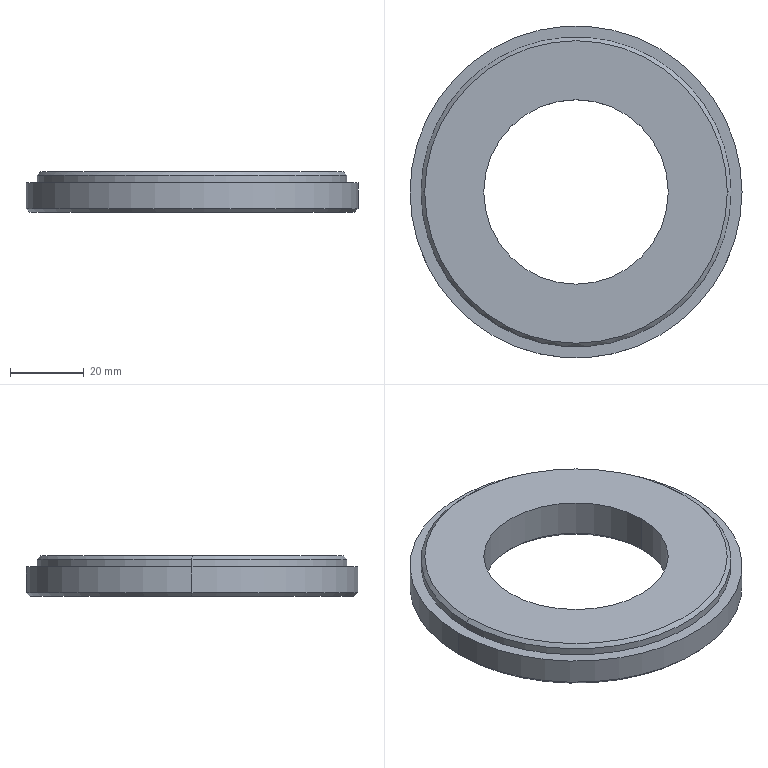Part | SolidWorks | features Chamfer 2, HoleWzd 1, ICE 1, Revolution 1 | 1 solid | 51 faces | box 90 x 90 x 11 mm | volume 45138 mm3 | cone 30 | cylinder 18 | plane 3 | commonest cylinder face diameters 3.3 x12 50 x2 84 x2 90 x2
STEP:
#1=CARTESIAN_POINT('',(-44.,0.,-11.));
#2=VERTEX_POINT('',#1);
#3=CARTESIAN_POINT('',(44.,0.,-11.));
#4=VERTEX_POINT('',#3);
#5=CARTESIAN_POINT('',(0.,0.,-11.));
#6=DIRECTION('',(0.,0.,-1.));
#7=DIRECTION('',(-1.,0.,0.));
#8=AXIS2_PLACEMENT_3D('',#5,#6,#7);
#9=CIRCLE('',#8,44.);
#10=EDGE_CURVE('',#2,#4,#9,.T.);
#11=ORIENTED_EDGE('',*,*,#10,.F.);
#12=CARTESIAN_POINT('',(-45.,0.,-10.));
#13=VERTEX_POINT('',#12);
#14=CARTESIAN_POINT('',(-45.,0.,-10.));
#15=DIRECTION('',(-0.7071,0.,0.7071));
#16=VECTOR('',#15,1000.);
#17=LINE('',#14,#16);
#18=EDGE_CURVE('',#2,#13,#17,.T.);
#19=ORIENTED_EDGE('',*,*,#18,.T.);
#20=CARTESIAN_POINT('',(45.,0.,-10.));
#21=VERTEX_POINT('',#20);
#22=CARTESIAN_POINT('',(0.,0.,-10.));
#23=DIRECTION('',(0.,0.,1.));
#24=DIRECTION('',(-1.,0.,0.));
#25=AXIS2_PLACEMENT_3D('',#22,#23,#24);
#26=CIRCLE('',#25,45.);
#27=EDGE_CURVE('',#21,#13,#26,.T.);
#28=ORIENTED_EDGE('',*,*,#27,.F.);
#29=CARTESIAN_POINT('',(45.,0.,-10.));
#30=DIRECTION('',(0.7071,0.,0.7071));
#31=VECTOR('',#30,1000.);
#32=LINE('',#29,#31);
#33=EDGE_CURVE('',#4,#21,#32,.T.);
#34=ORIENTED_EDGE('',*,*,#33,.F.);
#35=EDGE_LOOP('',(#11,#19,#28,#34));
#36=FACE_OUTER_BOUND('',#35,.T.);
#37=CARTESIAN_POINT('',(0.,0.,-10.));
#38=DIRECTION('',(0.,0.,1.));
#39=DIRECTION('',(1.,0.,0.));
#40=AXIS2_PLACEMENT_3D('',#37,#38,#39);
#41=CONICAL_SURFACE('',#40,45.,0.7854);
#42=ADVANCED_FACE('',(#36),#41,.T.);
#43=CARTESIAN_POINT('',(25.,0.,-10.));
#44=VERTEX_POINT('',#43);
#45=CARTESIAN_POINT('',(-25.,0.,-10.));
#46=VERTEX_POINT('',#45);
#47=CARTESIAN_POINT('',(0.,0.,-10.));
#48=DIRECTION('',(0.,0.,-1.));
#49=DIRECTION('',(-1.,0.,0.));
#50=AXIS2_PLACEMENT_3D('',#47,#48,#49);
#51=CIRCLE('',#50,25.);
#52=EDGE_CURVE('',#44,#46,#51,.T.);
#53=ORIENTED_EDGE('',*,*,#52,.F.);
#54=CARTESIAN_POINT('',(26.,0.,-11.));
#55=VERTEX_POINT('',#54);
#56=CARTESIAN_POINT('',(26.,0.,-11.));
#57=DIRECTION('',(0.7071,0.,-0.7071));
#58=VECTOR('',#57,1000.);
#59=LINE('',#56,#58);
#60=EDGE_CURVE('',#44,#55,#59,.T.);
#61=ORIENTED_EDGE('',*,*,#60,.T.);
#62=CARTESIAN_POINT('',(-26.,0.,-11.));
#63=VERTEX_POINT('',#62);
#64=CARTESIAN_POINT('',(0.,0.,-11.));
#65=DIRECTION('',(0.,0.,1.));
#66=DIRECTION('',(-1.,0.,0.));
#67=AXIS2_PLACEMENT_3D('',#64,#65,#66);
#68=CIRCLE('',#67,26.);
#69=EDGE_CURVE('',#63,#55,#68,.T.);
#70=ORIENTED_EDGE('',*,*,#69,.F.);
#71=CARTESIAN_POINT('',(-26.,0.,-11.));
#72=DIRECTION('',(-0.7071,0.,-0.7071));
#73=VECTOR('',#72,1000.);
#74=LINE('',#71,#73);
#75=EDGE_CURVE('',#46,#63,#74,.T.);
#76=ORIENTED_EDGE('',*,*,#75,.F.);
#77=EDGE_LOOP('',(#53,#61,#70,#76));
#78=FACE_OUTER_BOUND('',#77,.T.);
#79=CARTESIAN_POINT('',(0.,0.,-11.));
#80=DIRECTION('',(0.,0.,-1.));
#81=DIRECTION('',(-1.,0.,0.));
#82=AXIS2_PLACEMENT_3D('',#79,#80,#81);
#83=CONICAL_SURFACE('',#82,26.,0.7854);
#84=ADVANCED_FACE('',(#78),#83,.F.);
#85=CARTESIAN_POINT('',(41.,0.,0.));
#86=VERTEX_POINT('',#85);
#87=CARTESIAN_POINT('',(-41.,0.,0.));
#88=VERTEX_POINT('',#87);
#89=CARTESIAN_POINT('',(0.,0.,0.));
#90=DIRECTION('',(0.,0.,1.));
#91=DIRECTION('',(1.,0.,0.));
#92=AXIS2_PLACEMENT_3D('',#89,#90,#91);
#93=CIRCLE('',#92,41.);
#94=EDGE_CURVE('',#86,#88,#93,.T.);
#95=ORIENTED_EDGE('',*,*,#94,.F.);
#96=CARTESIAN_POINT('',(42.,0.,-1.));
#97=VERTEX_POINT('',#96);
#98=CARTESIAN_POINT('',(41.,0.,0.));
#99=DIRECTION('',(0.7071,0.,-0.7071));
#100=VECTOR('',#99,1000.);
#101=LINE('',#98,#100);
#102=EDGE_CURVE('',#86,#97,#101,.T.);
#103=ORIENTED_EDGE('',*,*,#102,.T.);
#104=CARTESIAN_POINT('',(-42.,0.,-1.));
#105=VERTEX_POINT('',#104);
#106=CARTESIAN_POINT('',(0.,0.,-1.));
#107=DIRECTION('',(0.,0.,-1.));
#108=DIRECTION('',(1.,0.,0.));
#109=AXIS2_PLACEMENT_3D('',#106,#107,#108);
#110=CIRCLE('',#109,42.);
#111=EDGE_CURVE('',#105,#97,#110,.T.);
#112=ORIENTED_EDGE('',*,*,#111,.F.);
#113=CARTESIAN_POINT('',(-41.,0.,0.));
#114=DIRECTION('',(-0.7071,0.,-0.7071));
#115=VECTOR('',#114,1000.);
#116=LINE('',#113,#115);
#117=EDGE_CURVE('',#88,#105,#116,.T.);
#118=ORIENTED_EDGE('',*,*,#117,.F.);
#119=EDGE_LOOP('',(#95,#103,#112,#118));
#120=FACE_OUTER_BOUND('',#119,.T.);
#121=CARTESIAN_POINT('',(0.,0.,0.));
#122=DIRECTION('',(0.,0.,-1.));
#123=DIRECTION('',(-1.,0.,0.));
#124=AXIS2_PLACEMENT_3D('',#121,#122,#123);
#125=CONICAL_SURFACE('',#124,41.,0.7854);
#126=ADVANCED_FACE('',(#120),#125,.T.);
#127=CARTESIAN_POINT('',(1.65,37.,-10.625));
#128=VERTEX_POINT('',#127);
#129=CARTESIAN_POINT('',(-1.65,37.,-10.625));
#130=VERTEX_POINT('',#129);
#131=CARTESIAN_POINT('',(0.,37.,-10.625));
#132=DIRECTION('',(0.,0.,-1.));
#133=DIRECTION('',(-1.,0.,0.));
#134=AXIS2_PLACEMENT_3D('',#131,#132,#133);
#135=CIRCLE('',#134,1.65);
#136=EDGE_CURVE('',#128,#130,#135,.T.);
#137=ORIENTED_EDGE('',*,*,#136,.F.);
#138=CARTESIAN_POINT('',(2.025,37.,-11.));
#139=VERTEX_POINT('',#138);
#140=CARTESIAN_POINT('',(1.65,37.,-10.625));
#141=DIRECTION('',(0.7071,0.,-0.7071));
#142=VECTOR('',#141,1000.);
#143=LINE('',#140,#142);
#144=EDGE_CURVE('',#128,#139,#143,.T.);
#145=ORIENTED_EDGE('',*,*,#144,.T.);
#146=CARTESIAN_POINT('',(-2.025,37.,-11.));
#147=VERTEX_POINT('',#146);
#148=CARTESIAN_POINT('',(0.,37.,-11.));
#149=DIRECTION('',(0.,0.,1.));
#150=DIRECTION('',(-1.,0.,0.));
#151=AXIS2_PLACEMENT_3D('',#148,#149,#150);
#152=CIRCLE('',#151,2.025);
#153=EDGE_CURVE('',#147,#139,#152,.T.);
#154=ORIENTED_EDGE('',*,*,#153,.F.);
#155=CARTESIAN_POINT('',(-1.65,37.,-10.625));
#156=DIRECTION('',(-0.7071,0.,-0.7071));
#157=VECTOR('',#156,1000.);
#158=LINE('',#155,#157);
#159=EDGE_CURVE('',#130,#147,#158,.T.);
#160=ORIENTED_EDGE('',*,*,#159,.F.);
#161=EDGE_LOOP('',(#137,#145,#154,#160));
#162=FACE_OUTER_BOUND('',#161,.T.);
#163=CARTESIAN_POINT('',(0.,37.,-10.625));
#164=DIRECTION('',(0.,0.,-1.));
#165=DIRECTION('',(-1.,0.,0.));
#166=AXIS2_PLACEMENT_3D('',#163,#164,#165);
#167=CONICAL_SURFACE('',#166,1.65,0.7854);
#168=ADVANCED_FACE('',(#162),#167,.F.);
#169=CARTESIAN_POINT('',(33.693,18.5,-10.625));
#170=VERTEX_POINT('',#169);
#171=CARTESIAN_POINT('',(30.393,18.5,-10.625));
#172=VERTEX_POINT('',#171);
#173=CARTESIAN_POINT('',(32.043,18.5,-10.625));
#174=DIRECTION('',(0.,0.,-1.));
#175=DIRECTION('',(-1.,0.,0.));
#176=AXIS2_PLACEMENT_3D('',#173,#174,#175);
#177=CIRCLE('',#176,1.65);
#178=EDGE_CURVE('',#170,#172,#177,.T.);
#179=ORIENTED_EDGE('',*,*,#178,.F.);
#180=CARTESIAN_POINT('',(34.068,18.5,-11.));
#181=VERTEX_POINT('',#180);
#182=CARTESIAN_POINT('',(33.693,18.5,-10.625));
#183=DIRECTION('',(0.7071,0.,-0.7071));
#184=VECTOR('',#183,1000.);
#185=LINE('',#182,#184);
#186=EDGE_CURVE('',#170,#181,#185,.T.);
#187=ORIENTED_EDGE('',*,*,#186,.T.);
#188=CARTESIAN_POINT('',(30.018,18.5,-11.));
#189=VERTEX_POINT('',#188);
#190=CARTESIAN_POINT('',(32.043,18.5,-11.));
#191=DIRECTION('',(0.,0.,1.));
#192=DIRECTION('',(-1.,0.,0.));
#193=AXIS2_PLACEMENT_3D('',#190,#191,#192);
#194=CIRCLE('',#193,2.025);
#195=EDGE_CURVE('',#189,#181,#194,.T.);
#196=ORIENTED_EDGE('',*,*,#195,.F.);
#197=CARTESIAN_POINT('',(30.393,18.5,-10.625));
#198=DIRECTION('',(-0.7071,0.,-0.7071));
#199=VECTOR('',#198,1000.);
#200=LINE('',#197,#199);
#201=EDGE_CURVE('',#172,#189,#200,.T.);
#202=ORIENTED_EDGE('',*,*,#201,.F.);
#203=EDGE_LOOP('',(#179,#187,#196,#202));
#204=FACE_OUTER_BOUND('',#203,.T.);
#205=CARTESIAN_POINT('',(32.043,18.5,-10.625));
#206=DIRECTION('',(0.,0.,-1.));
#207=DIRECTION('',(-1.,0.,0.));
#208=AXIS2_PLACEMENT_3D('',#205,#206,#207);
#209=CONICAL_SURFACE('',#208,1.65,0.7854);
#210=ADVANCED_FACE('',(#204),#209,.F.);
#211=CARTESIAN_POINT('',(33.693,-18.5,-10.625));
#212=VERTEX_POINT('',#211);
#213=CARTESIAN_POINT('',(30.393,-18.5,-10.625));
#214=VERTEX_POINT('',#213);
#215=CARTESIAN_POINT('',(32.043,-18.5,-10.625));
#216=DIRECTION('',(0.,0.,-1.));
#217=DIRECTION('',(-1.,0.,0.));
#218=AXIS2_PLACEMENT_3D('',#215,#216,#217);
#219=CIRCLE('',#218,1.65);
#220=EDGE_CURVE('',#212,#214,#219,.T.);
#221=ORIENTED_EDGE('',*,*,#220,.F.);
#222=CARTESIAN_POINT('',(34.068,-18.5,-11.));
#223=VERTEX_POINT('',#222);
#224=CARTESIAN_POINT('',(33.693,-18.5,-10.625));
#225=DIRECTION('',(0.7071,0.,-0.7071));
#226=VECTOR('',#225,1000.);
#227=LINE('',#224,#226);
#228=EDGE_CURVE('',#212,#223,#227,.T.);
#229=ORIENTED_EDGE('',*,*,#228,.T.);
#230=CARTESIAN_POINT('',(30.018,-18.5,-11.));
#231=VERTEX_POINT('',#230);
#232=CARTESIAN_POINT('',(32.043,-18.5,-11.));
#233=DIRECTION('',(0.,0.,1.));
#234=DIRECTION('',(-1.,0.,0.));
#235=AXIS2_PLACEMENT_3D('',#232,#233,#234);
#236=CIRCLE('',#235,2.025);
#237=EDGE_CURVE('',#231,#223,#236,.T.);
#238=ORIENTED_EDGE('',*,*,#237,.F.);
#239=CARTESIAN_POINT('',(30.393,-18.5,-10.625));
#240=DIRECTION('',(-0.7071,0.,-0.7071));
#241=VECTOR('',#240,1000.);
#242=LINE('',#239,#241);
#243=EDGE_CURVE('',#214,#231,#242,.T.);
#244=ORIENTED_EDGE('',*,*,#243,.F.);
#245=EDGE_LOOP('',(#221,#229,#238,#244));
#246=FACE_OUTER_BOUND('',#245,.T.);
#247=CARTESIAN_POINT('',(32.043,-18.5,-10.625));
#248=DIRECTION('',(0.,0.,-1.));
#249=DIRECTION('',(-1.,0.,0.));
#250=AXIS2_PLACEMENT_3D('',#247,#248,#249);
#251=CONICAL_SURFACE('',#250,1.65,0.7854);
#252=ADVANCED_FACE('',(#246),#251,.F.);
#253=CARTESIAN_POINT('',(1.65,-37.,-10.625));
#254=VERTEX_POINT('',#253);
#255=CARTESIAN_POINT('',(-1.65,-37.,-10.625));
#256=VERTEX_POINT('',#255);
#257=CARTESIAN_POINT('',(0.,-37.,-10.625));
#258=DIRECTION('',(0.,0.,-1.));
#259=DIRECTION('',(-1.,0.,0.));
#260=AXIS2_PLACEMENT_3D('',#257,#258,#259);
#261=CIRCLE('',#260,1.65);
#262=EDGE_CURVE('',#254,#256,#261,.T.);
#263=ORIENTED_EDGE('',*,*,#262,.F.);
#264=CARTESIAN_POINT('',(2.025,-37.,-11.));
#265=VERTEX_POINT('',#264);
#266=CARTESIAN_POINT('',(1.65,-37.,-10.625));
#267=DIRECTION('',(0.7071,0.,-0.7071));
#268=VECTOR('',#267,1000.);
#269=LINE('',#266,#268);
#270=EDGE_CURVE('',#254,#265,#269,.T.);
#271=ORIENTED_EDGE('',*,*,#270,.T.);
#272=CARTESIAN_POINT('',(-2.025,-37.,-11.));
#273=VERTEX_POINT('',#272);
#274=CARTESIAN_POINT('',(0.,-37.,-11.));
#275=DIRECTION('',(0.,0.,1.));
#276=DIRECTION('',(-1.,0.,0.));
#277=AXIS2_PLACEMENT_3D('',#274,#275,#276);
#278=CIRCLE('',#277,2.025);
#279=EDGE_CURVE('',#273,#265,#278,.T.);
#280=ORIENTED_EDGE('',*,*,#279,.F.);
#281=CARTESIAN_POINT('',(-1.65,-37.,-10.625));
#282=DIRECTION('',(-0.7071,0.,-0.7071));
#283=VECTOR('',#282,1000.);
#284=LINE('',#281,#283);
#285=EDGE_CURVE('',#256,#273,#284,.T.);
#286=ORIENTED_EDGE('',*,*,#285,.F.);
#287=EDGE_LOOP('',(#263,#271,#280,#286));
#288=FACE_OUTER_BOUND('',#287,.T.);
#289=CARTESIAN_POINT('',(0.,-37.,-10.625));
#290=DIRECTION('',(0.,0.,-1.));
#291=DIRECTION('',(-1.,0.,0.));
#292=AXIS2_PLACEMENT_3D('',#289,#290,#291);
#293=CONICAL_SURFACE('',#292,1.65,0.7854);
#294=ADVANCED_FACE('',(#288),#293,.F.);
#295=CARTESIAN_POINT('',(-30.393,-18.5,-10.625));
#296=VERTEX_POINT('',#295);
#297=CARTESIAN_POINT('',(-33.693,-18.5,-10.625));
#298=VERTEX_POINT('',#297);
#299=CARTESIAN_POINT('',(-32.043,-18.5,-10.625));
#300=DIRECTION('',(0.,0.,-1.));
#301=DIRECTION('',(-1.,0.,0.));
#302=AXIS2_PLACEMENT_3D('',#299,#300,#301);
#303=CIRCLE('',#302,1.65);
#304=EDGE_CURVE('',#296,#298,#303,.T.);
#305=ORIENTED_EDGE('',*,*,#304,.F.);
#306=CARTESIAN_POINT('',(-30.018,-18.5,-11.));
#307=VERTEX_POINT('',#306);
#308=CARTESIAN_POINT('',(-30.393,-18.5,-10.625));
#309=DIRECTION('',(0.7071,0.,-0.7071));
#310=VECTOR('',#309,1000.);
#311=LINE('',#308,#310);
#312=EDGE_CURVE('',#296,#307,#311,.T.);
#313=ORIENTED_EDGE('',*,*,#312,.T.);
#314=CARTESIAN_POINT('',(-34.068,-18.5,-11.));
#315=VERTEX_POINT('',#314);
#316=CARTESIAN_POINT('',(-32.043,-18.5,-11.));
#317=DIRECTION('',(0.,0.,1.));
#318=DIRECTION('',(-1.,0.,0.));
#319=AXIS2_PLACEMENT_3D('',#316,#317,#318);
#320=CIRCLE('',#319,2.025);
#321=EDGE_CURVE('',#315,#307,#320,.T.);
#322=ORIENTED_EDGE('',*,*,#321,.F.);
#323=CARTESIAN_POINT('',(-33.693,-18.5,-10.625));
#324=DIRECTION('',(-0.7071,0.,-0.7071));
#325=VECTOR('',#324,1000.);
#326=LINE('',#323,#325);
#327=EDGE_CURVE('',#298,#315,#326,.T.);
#328=ORIENTED_EDGE('',*,*,#327,.F.);
#329=EDGE_LOOP('',(#305,#313,#322,#328));
#330=FACE_OUTER_BOUND('',#329,.T.);
#331=CARTESIAN_POINT('',(-32.043,-18.5,-10.625));
#332=DIRECTION('',(0.,0.,-1.));
#333=DIRECTION('',(-1.,0.,0.));
#334=AXIS2_PLACEMENT_3D('',#331,#332,#333);
#335=CONICAL_SURFACE('',#334,1.65,0.7854);
#336=ADVANCED_FACE('',(#330),#335,.F.);
#337=CARTESIAN_POINT('',(-30.393,18.5,-10.625));
#338=VERTEX_POINT('',#337);
#339=CARTESIAN_POINT('',(-33.693,18.5,-10.625));
#340=VERTEX_POINT('',#339);
#341=CARTESIAN_POINT('',(-32.043,18.5,-10.625));
#342=DIRECTION('',(0.,0.,-1.));
#343=DIRECTION('',(-1.,0.,0.));
#344=AXIS2_PLACEMENT_3D('',#341,#342,#343);
#345=CIRCLE('',#344,1.65);
#346=EDGE_CURVE('',#338,#340,#345,.T.);
#347=ORIENTED_EDGE('',*,*,#346,.F.);
#348=CARTESIAN_POINT('',(-30.018,18.5,-11.));
#349=VERTEX_POINT('',#348);
#350=CARTESIAN_POINT('',(-30.393,18.5,-10.625));
#351=DIRECTION('',(0.7071,0.,-0.7071));
#352=VECTOR('',#351,1000.);
#353=LINE('',#350,#352);
#354=EDGE_CURVE('',#338,#349,#353,.T.);
#355=ORIENTED_EDGE('',*,*,#354,.T.);
#356=CARTESIAN_POINT('',(-34.068,18.5,-11.));
#357=VERTEX_POINT('',#356);
#358=CARTESIAN_POINT('',(-32.043,18.5,-11.));
#359=DIRECTION('',(0.,0.,1.));
#360=DIRECTION('',(-1.,0.,0.));
#361=AXIS2_PLACEMENT_3D('',#358,#359,#360);
#362=CIRCLE('',#361,2.025);
#363=EDGE_CURVE('',#357,#349,#362,.T.);
#364=ORIENTED_EDGE('',*,*,#363,.F.);
#365=CARTESIAN_POINT('',(-33.693,18.5,-10.625));
#366=DIRECTION('',(-0.7071,0.,-0.7071));
#367=VECTOR('',#366,1000.);
#368=LINE('',#365,#367);
#369=EDGE_CURVE('',#340,#357,#368,.T.);
#370=ORIENTED_EDGE('',*,*,#369,.F.);
#371=EDGE_LOOP('',(#347,#355,#364,#370));
#372=FACE_OUTER_BOUND('',#371,.T.);
#373=CARTESIAN_POINT('',(-32.043,18.5,-10.625));
#374=DIRECTION('',(0.,0.,-1.));
#375=DIRECTION('',(-1.,0.,0.));
#376=AXIS2_PLACEMENT_3D('',#373,#374,#375);
#377=CONICAL_SURFACE('',#376,1.65,0.7854);
#378=ADVANCED_FACE('',(#372),#377,.F.);
#379=CARTESIAN_POINT('',(1.65,-37.,-3.));
#380=VERTEX_POINT('',#379);
#381=CARTESIAN_POINT('',(-1.65,-37.,-3.));
#382=VERTEX_POINT('',#381);
#383=CARTESIAN_POINT('',(0.,-37.,-3.));
#384=DIRECTION('',(0.,0.,-1.));
#385=DIRECTION('',(-1.,0.,0.));
#386=AXIS2_PLACEMENT_3D('',#383,#384,#385);
#387=CIRCLE('',#386,1.65);
#388=EDGE_CURVE('',#380,#382,#387,.T.);
#389=ORIENTED_EDGE('',*,*,#388,.F.);
#390=CARTESIAN_POINT('',(1.65,-37.,-11.));
#391=DIRECTION('',(0.,0.,-1.));
#392=VECTOR('',#391,1000.);
#393=LINE('',#390,#392);
#394=EDGE_CURVE('',#380,#254,#393,.T.);
#395=ORIENTED_EDGE('',*,*,#394,.T.);
#396=ORIENTED_EDGE('',*,*,#262,.T.);
#397=CARTESIAN_POINT('',(-1.65,-37.,-11.));
#398=DIRECTION('',(0.,0.,-1.));
#399=VECTOR('',#398,1000.);
#400=LINE('',#397,#399);
#401=EDGE_CURVE('',#382,#256,#400,.T.);
#402=ORIENTED_EDGE('',*,*,#401,.F.);
#403=EDGE_LOOP('',(#389,#395,#396,#402));
#404=FACE_OUTER_BOUND('',#403,.T.);
#405=CARTESIAN_POINT('',(0.,-37.,-11.));
#406=DIRECTION('',(0.,0.,-1.));
#407=DIRECTION('',(-1.,0.,0.));
#408=AXIS2_PLACEMENT_3D('',#405,#406,#407);
#409=CYLINDRICAL_SURFACE('',#408,1.65);
#410=ADVANCED_FACE('',(#404),#409,.F.);
#411=CARTESIAN_POINT('',(0.,-37.,-2.009));
#412=VERTEX_POINT('',#411);
#413=CARTESIAN_POINT('',(-1.65,-37.,-3.));
#414=DIRECTION('',(-0.8572,0.,-0.515));
#415=VECTOR('',#414,1000.);
#416=LINE('',#413,#415);
#417=EDGE_CURVE('',#412,#382,#416,.T.);
#418=ORIENTED_EDGE('',*,*,#417,.F.);
#419=CARTESIAN_POINT('',(1.65,-37.,-3.));
#420=DIRECTION('',(0.8572,0.,-0.515));
#421=VECTOR('',#420,1000.);
#422=LINE('',#419,#421);
#423=EDGE_CURVE('',#412,#380,#422,.T.);
#424=ORIENTED_EDGE('',*,*,#423,.T.);
#425=ORIENTED_EDGE('',*,*,#388,.T.);
#426=EDGE_LOOP('',(#418,#424,#425));
#427=FACE_OUTER_BOUND('',#426,.T.);
#428=CARTESIAN_POINT('',(0.,-37.,-3.));
#429=DIRECTION('',(0.,0.,-1.));
#430=DIRECTION('',(-1.,0.,0.));
#431=AXIS2_PLACEMENT_3D('',#428,#429,#430);
#432=CONICAL_SURFACE('',#431,1.65,1.03);
#433=ADVANCED_FACE('',(#427),#432,.F.);
#434=CARTESIAN_POINT('',(33.693,-18.5,-3.));
#435=VERTEX_POINT('',#434);
#436=CARTESIAN_POINT('',(30.393,-18.5,-3.));
#437=VERTEX_POINT('',#436);
#438=CARTESIAN_POINT('',(32.043,-18.5,-3.));
#439=DIRECTION('',(0.,0.,-1.));
#440=DIRECTION('',(-1.,0.,0.));
#441=AXIS2_PLACEMENT_3D('',#438,#439,#440);
#442=CIRCLE('',#441,1.65);
#443=EDGE_CURVE('',#435,#437,#442,.T.);
#444=ORIENTED_EDGE('',*,*,#443,.F.);
#445=CARTESIAN_POINT('',(33.693,-18.5,-11.));
#446=DIRECTION('',(0.,0.,-1.));
#447=VECTOR('',#446,1000.);
#448=LINE('',#445,#447);
#449=EDGE_CURVE('',#435,#212,#448,.T.);
#450=ORIENTED_EDGE('',*,*,#449,.T.);
#451=ORIENTED_EDGE('',*,*,#220,.T.);
#452=CARTESIAN_POINT('',(30.393,-18.5,-11.));
#453=DIRECTION('',(0.,0.,-1.));
#454=VECTOR('',#453,1000.);
#455=LINE('',#452,#454);
#456=EDGE_CURVE('',#437,#214,#455,.T.);
#457=ORIENTED_EDGE('',*,*,#456,.F.);
#458=EDGE_LOOP('',(#444,#450,#451,#457));
#459=FACE_OUTER_BOUND('',#458,.T.);
#460=CARTESIAN_POINT('',(32.043,-18.5,-11.));
#461=DIRECTION('',(0.,0.,-1.));
#462=DIRECTION('',(-1.,0.,0.));
#463=AXIS2_PLACEMENT_3D('',#460,#461,#462);
#464=CYLINDRICAL_SURFACE('',#463,1.65);
#465=ADVANCED_FACE('',(#459),#464,.F.);
#466=CARTESIAN_POINT('',(32.043,-18.5,-2.009));
#467=VERTEX_POINT('',#466);
#468=CARTESIAN_POINT('',(30.393,-18.5,-3.));
#469=DIRECTION('',(-0.8572,0.,-0.515));
#470=VECTOR('',#469,1000.);
#471=LINE('',#468,#470);
#472=EDGE_CURVE('',#467,#437,#471,.T.);
#473=ORIENTED_EDGE('',*,*,#472,.F.);
#474=CARTESIAN_POINT('',(33.693,-18.5,-3.));
#475=DIRECTION('',(0.8572,0.,-0.515));
#476=VECTOR('',#475,1000.);
#477=LINE('',#474,#476);
#478=EDGE_CURVE('',#467,#435,#477,.T.);
#479=ORIENTED_EDGE('',*,*,#478,.T.);
#480=ORIENTED_EDGE('',*,*,#443,.T.);
#481=EDGE_LOOP('',(#473,#479,#480));
#482=FACE_OUTER_BOUND('',#481,.T.);
#483=CARTESIAN_POINT('',(32.043,-18.5,-3.));
#484=DIRECTION('',(0.,0.,-1.));
#485=DIRECTION('',(-1.,0.,0.));
#486=AXIS2_PLACEMENT_3D('',#483,#484,#485);
#487=CONICAL_SURFACE('',#486,1.65,1.03);
#488=ADVANCED_FACE('',(#482),#487,.F.);
#489=CARTESIAN_POINT('',(33.693,18.5,-3.));
#490=VERTEX_POINT('',#489);
#491=CARTESIAN_POINT('',(30.393,18.5,-3.));
#492=VERTEX_POINT('',#491);
#493=CARTESIAN_POINT('',(32.043,18.5,-3.));
#494=DIRECTION('',(0.,0.,-1.));
#495=DIRECTION('',(-1.,0.,0.));
#496=AXIS2_PLACEMENT_3D('',#493,#494,#495);
#497=CIRCLE('',#496,1.65);
#498=EDGE_CURVE('',#490,#492,#497,.T.);
#499=ORIENTED_EDGE('',*,*,#498,.F.);
#500=CARTESIAN_POINT('',(33.693,18.5,-11.));
#501=DIRECTION('',(0.,0.,-1.));
#502=VECTOR('',#501,1000.);
#503=LINE('',#500,#502);
#504=EDGE_CURVE('',#490,#170,#503,.T.);
#505=ORIENTED_EDGE('',*,*,#504,.T.);
#506=ORIENTED_EDGE('',*,*,#178,.T.);
#507=CARTESIAN_POINT('',(30.393,18.5,-11.));
#508=DIRECTION('',(0.,0.,-1.));
#509=VECTOR('',#508,1000.);
#510=LINE('',#507,#509);
#511=EDGE_CURVE('',#492,#172,#510,.T.);
#512=ORIENTED_EDGE('',*,*,#511,.F.);
#513=EDGE_LOOP('',(#499,#505,#506,#512));
#514=FACE_OUTER_BOUND('',#513,.T.);
#515=CARTESIAN_POINT('',(32.043,18.5,-11.));
#516=DIRECTION('',(0.,0.,-1.));
#517=DIRECTION('',(-1.,0.,0.));
#518=AXIS2_PLACEMENT_3D('',#515,#516,#517);
#519=CYLINDRICAL_SURFACE('',#518,1.65);
#520=ADVANCED_FACE('',(#514),#519,.F.);
#521=CARTESIAN_POINT('',(32.043,18.5,-2.009));
#522=VERTEX_POINT('',#521);
#523=CARTESIAN_POINT('',(30.393,18.5,-3.));
#524=DIRECTION('',(-0.8572,0.,-0.515));
#525=VECTOR('',#524,1000.);
#526=LINE('',#523,#525);
#527=EDGE_CURVE('',#522,#492,#526,.T.);
#528=ORIENTED_EDGE('',*,*,#527,.F.);
#529=CARTESIAN_POINT('',(33.693,18.5,-3.));
#530=DIRECTION('',(0.8572,0.,-0.515));
#531=VECTOR('',#530,1000.);
#532=LINE('',#529,#531);
#533=EDGE_CURVE('',#522,#490,#532,.T.);
#534=ORIENTED_EDGE('',*,*,#533,.T.);
#535=ORIENTED_EDGE('',*,*,#498,.T.);
#536=EDGE_LOOP('',(#528,#534,#535));
#537=FACE_OUTER_BOUND('',#536,.T.);
#538=CARTESIAN_POINT('',(32.043,18.5,-3.));
#539=DIRECTION('',(0.,0.,-1.));
#540=DIRECTION('',(-1.,0.,0.));
#541=AXIS2_PLACEMENT_3D('',#538,#539,#540);
#542=CONICAL_SURFACE('',#541,1.65,1.03);
#543=ADVANCED_FACE('',(#537),#542,.F.);
#544=CARTESIAN_POINT('',(1.65,37.,-3.));
#545=VERTEX_POINT('',#544);
#546=CARTESIAN_POINT('',(-1.65,37.,-3.));
#547=VERTEX_POINT('',#546);
#548=CARTESIAN_POINT('',(0.,37.,-3.));
#549=DIRECTION('',(0.,0.,-1.));
#550=DIRECTION('',(-1.,0.,0.));
#551=AXIS2_PLACEMENT_3D('',#548,#549,#550);
#552=CIRCLE('',#551,1.65);
#553=EDGE_CURVE('',#545,#547,#552,.T.);
#554=ORIENTED_EDGE('',*,*,#553,.F.);
#555=CARTESIAN_POINT('',(1.65,37.,-11.));
#556=DIRECTION('',(0.,0.,-1.));
#557=VECTOR('',#556,1000.);
#558=LINE('',#555,#557);
#559=EDGE_CURVE('',#545,#128,#558,.T.);
#560=ORIENTED_EDGE('',*,*,#559,.T.);
#561=ORIENTED_EDGE('',*,*,#136,.T.);
#562=CARTESIAN_POINT('',(-1.65,37.,-11.));
#563=DIRECTION('',(0.,0.,-1.));
#564=VECTOR('',#563,1000.);
#565=LINE('',#562,#564);
#566=EDGE_CURVE('',#547,#130,#565,.T.);
#567=ORIENTED_EDGE('',*,*,#566,.F.);
#568=EDGE_LOOP('',(#554,#560,#561,#567));
#569=FACE_OUTER_BOUND('',#568,.T.);
#570=CARTESIAN_POINT('',(0.,37.,-11.));
#571=DIRECTION('',(0.,0.,-1.));
#572=DIRECTION('',(-1.,0.,0.));
#573=AXIS2_PLACEMENT_3D('',#570,#571,#572);
#574=CYLINDRICAL_SURFACE('',#573,1.65);
#575=ADVANCED_FACE('',(#569),#574,.F.);
#576=CARTESIAN_POINT('',(0.,37.,-2.009));
#577=VERTEX_POINT('',#576);
#578=CARTESIAN_POINT('',(-1.65,37.,-3.));
#579=DIRECTION('',(-0.8572,0.,-0.515));
#580=VECTOR('',#579,1000.);
#581=LINE('',#578,#580);
#582=EDGE_CURVE('',#577,#547,#581,.T.);
#583=ORIENTED_EDGE('',*,*,#582,.F.);
#584=CARTESIAN_POINT('',(1.65,37.,-3.));
#585=DIRECTION('',(0.8572,0.,-0.515));
#586=VECTOR('',#585,1000.);
#587=LINE('',#584,#586);
#588=EDGE_CURVE('',#577,#545,#587,.T.);
#589=ORIENTED_EDGE('',*,*,#588,.T.);
#590=ORIENTED_EDGE('',*,*,#553,.T.);
#591=EDGE_LOOP('',(#583,#589,#590));
#592=FACE_OUTER_BOUND('',#591,.T.);
#593=CARTESIAN_POINT('',(0.,37.,-3.));
#594=DIRECTION('',(0.,0.,-1.));
#595=DIRECTION('',(-1.,0.,0.));
#596=AXIS2_PLACEMENT_3D('',#593,#594,#595);
#597=CONICAL_SURFACE('',#596,1.65,1.03);
#598=ADVANCED_FACE('',(#592),#597,.F.);
#599=CARTESIAN_POINT('',(-30.393,-18.5,-3.));
#600=VERTEX_POINT('',#599);
#601=CARTESIAN_POINT('',(-33.693,-18.5,-3.));
#602=VERTEX_POINT('',#601);
#603=CARTESIAN_POINT('',(-32.043,-18.5,-3.));
#604=DIRECTION('',(0.,0.,-1.));
#605=DIRECTION('',(-1.,0.,0.));
#606=AXIS2_PLACEMENT_3D('',#603,#604,#605);
#607=CIRCLE('',#606,1.65);
#608=EDGE_CURVE('',#600,#602,#607,.T.);
#609=ORIENTED_EDGE('',*,*,#608,.F.);
#610=CARTESIAN_POINT('',(-30.393,-18.5,-11.));
#611=DIRECTION('',(0.,0.,-1.));
#612=VECTOR('',#611,1000.);
#613=LINE('',#610,#612);
#614=EDGE_CURVE('',#600,#296,#613,.T.);
#615=ORIENTED_EDGE('',*,*,#614,.T.);
#616=ORIENTED_EDGE('',*,*,#304,.T.);
#617=CARTESIAN_POINT('',(-33.693,-18.5,-11.));
#618=DIRECTION('',(0.,0.,-1.));
#619=VECTOR('',#618,1000.);
#620=LINE('',#617,#619);
#621=EDGE_CURVE('',#602,#298,#620,.T.);
#622=ORIENTED_EDGE('',*,*,#621,.F.);
#623=EDGE_LOOP('',(#609,#615,#616,#622));
#624=FACE_OUTER_BOUND('',#623,.T.);
#625=CARTESIAN_POINT('',(-32.043,-18.5,-11.));
#626=DIRECTION('',(0.,0.,-1.));
#627=DIRECTION('',(-1.,0.,0.));
#628=AXIS2_PLACEMENT_3D('',#625,#626,#627);
#629=CYLINDRICAL_SURFACE('',#628,1.65);
#630=ADVANCED_FACE('',(#624),#629,.F.);
#631=CARTESIAN_POINT('',(-32.043,-18.5,-2.009));
#632=VERTEX_POINT('',#631);
#633=CARTESIAN_POINT('',(-33.693,-18.5,-3.));
#634=DIRECTION('',(-0.8572,0.,-0.515));
#635=VECTOR('',#634,1000.);
#636=LINE('',#633,#635);
#637=EDGE_CURVE('',#632,#602,#636,.T.);
#638=ORIENTED_EDGE('',*,*,#637,.F.);
#639=CARTESIAN_POINT('',(-30.393,-18.5,-3.));
#640=DIRECTION('',(0.8572,0.,-0.515));
#641=VECTOR('',#640,1000.);
#642=LINE('',#639,#641);
#643=EDGE_CURVE('',#632,#600,#642,.T.);
#644=ORIENTED_EDGE('',*,*,#643,.T.);
#645=ORIENTED_EDGE('',*,*,#608,.T.);
#646=EDGE_LOOP('',(#638,#644,#645));
#647=FACE_OUTER_BOUND('',#646,.T.);
#648=CARTESIAN_POINT('',(-32.043,-18.5,-3.));
#649=DIRECTION('',(0.,0.,-1.));
#650=DIRECTION('',(-1.,0.,0.));
#651=AXIS2_PLACEMENT_3D('',#648,#649,#650);
#652=CONICAL_SURFACE('',#651,1.65,1.03);
#653=ADVANCED_FACE('',(#647),#652,.F.);
#654=CARTESIAN_POINT('',(-30.393,18.5,-3.));
#655=VERTEX_POINT('',#654);
#656=CARTESIAN_POINT('',(-33.693,18.5,-3.));
#657=VERTEX_POINT('',#656);
#658=CARTESIAN_POINT('',(-32.043,18.5,-3.));
#659=DIRECTION('',(0.,0.,-1.));
#660=DIRECTION('',(-1.,0.,0.));
#661=AXIS2_PLACEMENT_3D('',#658,#659,#660);
#662=CIRCLE('',#661,1.65);
#663=EDGE_CURVE('',#655,#657,#662,.T.);
#664=ORIENTED_EDGE('',*,*,#663,.F.);
#665=CARTESIAN_POINT('',(-30.393,18.5,-11.));
#666=DIRECTION('',(0.,0.,-1.));
#667=VECTOR('',#666,1000.);
#668=LINE('',#665,#667);
#669=EDGE_CURVE('',#655,#338,#668,.T.);
#670=ORIENTED_EDGE('',*,*,#669,.T.);
#671=ORIENTED_EDGE('',*,*,#346,.T.);
#672=CARTESIAN_POINT('',(-33.693,18.5,-11.));
#673=DIRECTION('',(0.,0.,-1.));
#674=VECTOR('',#673,1000.);
#675=LINE('',#672,#674);
#676=EDGE_CURVE('',#657,#340,#675,.T.);
#677=ORIENTED_EDGE('',*,*,#676,.F.);
#678=EDGE_LOOP('',(#664,#670,#671,#677));
#679=FACE_OUTER_BOUND('',#678,.T.);
#680=CARTESIAN_POINT('',(-32.043,18.5,-11.));
#681=DIRECTION('',(0.,0.,-1.));
#682=DIRECTION('',(-1.,0.,0.));
#683=AXIS2_PLACEMENT_3D('',#680,#681,#682);
#684=CYLINDRICAL_SURFACE('',#683,1.65);
#685=ADVANCED_FACE('',(#679),#684,.F.);
#686=CARTESIAN_POINT('',(-32.043,18.5,-2.009));
#687=VERTEX_POINT('',#686);
#688=CARTESIAN_POINT('',(-33.693,18.5,-3.));
#689=DIRECTION('',(-0.8572,0.,-0.515));
#690=VECTOR('',#689,1000.);
#691=LINE('',#688,#690);
#692=EDGE_CURVE('',#687,#657,#691,.T.);
#693=ORIENTED_EDGE('',*,*,#692,.F.);
#694=CARTESIAN_POINT('',(-30.393,18.5,-3.));
#695=DIRECTION('',(0.8572,0.,-0.515));
#696=VECTOR('',#695,1000.);
#697=LINE('',#694,#696);
#698=EDGE_CURVE('',#687,#655,#697,.T.);
#699=ORIENTED_EDGE('',*,*,#698,.T.);
#700=ORIENTED_EDGE('',*,*,#663,.T.);
#701=EDGE_LOOP('',(#693,#699,#700));
#702=FACE_OUTER_BOUND('',#701,.T.);
#703=CARTESIAN_POINT('',(-32.043,18.5,-3.));
#704=DIRECTION('',(0.,0.,-1.));
#705=DIRECTION('',(-1.,0.,0.));
#706=AXIS2_PLACEMENT_3D('',#703,#704,#705);
#707=CONICAL_SURFACE('',#706,1.65,1.03);
#708=ADVANCED_FACE('',(#702),#707,.F.);
#709=ORIENTED_EDGE('',*,*,#27,.T.);
#710=CARTESIAN_POINT('',(-45.,0.,-3.));
#711=VERTEX_POINT('',#710);
#712=CARTESIAN_POINT('',(-45.,0.,0.));
#713=DIRECTION('',(0.,0.,1.));
#714=VECTOR('',#713,1000.);
#715=LINE('',#712,#714);
#716=EDGE_CURVE('',#13,#711,#715,.T.);
#717=ORIENTED_EDGE('',*,*,#716,.T.);
#718=CARTESIAN_POINT('',(45.,0.,-3.));
#719=VERTEX_POINT('',#718);
#720=CARTESIAN_POINT('',(0.,0.,-3.));
#721=DIRECTION('',(0.,0.,1.));
#722=DIRECTION('',(1.,0.,0.));
#723=AXIS2_PLACEMENT_3D('',#720,#721,#722);
#724=CIRCLE('',#723,45.);
#725=EDGE_CURVE('',#719,#711,#724,.T.);
#726=ORIENTED_EDGE('',*,*,#725,.F.);
#727=CARTESIAN_POINT('',(45.,0.,0.));
#728=DIRECTION('',(0.,0.,1.));
#729=VECTOR('',#728,1000.);
#730=LINE('',#727,#729);
#731=EDGE_CURVE('',#21,#719,#730,.T.);
#732=ORIENTED_EDGE('',*,*,#731,.F.);
#733=EDGE_LOOP('',(#709,#717,#726,#732));
#734=FACE_OUTER_BOUND('',#733,.T.);
#735=CARTESIAN_POINT('',(0.,0.,0.));
#736=DIRECTION('',(0.,0.,1.));
#737=DIRECTION('',(1.,0.,0.));
#738=AXIS2_PLACEMENT_3D('',#735,#736,#737);
#739=CYLINDRICAL_SURFACE('',#738,45.);
#740=ADVANCED_FACE('',(#734),#739,.T.);
#741=CARTESIAN_POINT('',(42.,0.,-3.));
#742=VERTEX_POINT('',#741);
#743=CARTESIAN_POINT('',(-42.,0.,-3.));
#744=VERTEX_POINT('',#743);
#745=CARTESIAN_POINT('',(0.,0.,-3.));
#746=DIRECTION('',(0.,0.,1.));
#747=DIRECTION('',(1.,0.,0.));
#748=AXIS2_PLACEMENT_3D('',#745,#746,#747);
#749=CIRCLE('',#748,42.);
#750=EDGE_CURVE('',#742,#744,#749,.T.);
#751=ORIENTED_EDGE('',*,*,#750,.T.);
#752=CARTESIAN_POINT('',(-42.,0.,0.));
#753=DIRECTION('',(0.,0.,1.));
#754=VECTOR('',#753,1000.);
#755=LINE('',#752,#754);
#756=EDGE_CURVE('',#744,#105,#755,.T.);
#757=ORIENTED_EDGE('',*,*,#756,.T.);
#758=ORIENTED_EDGE('',*,*,#111,.T.);
#759=CARTESIAN_POINT('',(42.,0.,0.));
#760=DIRECTION('',(0.,0.,1.));
#761=VECTOR('',#760,1000.);
#762=LINE('',#759,#761);
#763=EDGE_CURVE('',#742,#97,#762,.T.);
#764=ORIENTED_EDGE('',*,*,#763,.F.);
#765=EDGE_LOOP('',(#751,#757,#758,#764));
#766=FACE_OUTER_BOUND('',#765,.T.);
#767=CARTESIAN_POINT('',(0.,0.,0.));
#768=DIRECTION('',(0.,0.,1.));
#769=DIRECTION('',(1.,0.,0.));
#770=AXIS2_PLACEMENT_3D('',#767,#768,#769);
#771=CYLINDRICAL_SURFACE('',#770,42.);
#772=ADVANCED_FACE('',(#766),#771,.T.);
#773=ORIENTED_EDGE('',*,*,#52,.T.);
#774=CARTESIAN_POINT('',(-25.,0.,0.));
#775=VERTEX_POINT('',#774);
#776=CARTESIAN_POINT('',(-25.,0.,0.));
#777=DIRECTION('',(0.,0.,1.));
#778=VECTOR('',#777,1000.);
#779=LINE('',#776,#778);
#780=EDGE_CURVE('',#46,#775,#779,.T.);
#781=ORIENTED_EDGE('',*,*,#780,.T.);
#782=CARTESIAN_POINT('',(25.,0.,0.));
#783=VERTEX_POINT('',#782);
#784=CARTESIAN_POINT('',(0.,0.,0.));
#785=DIRECTION('',(0.,0.,1.));
#786=DIRECTION('',(1.,0.,0.));
#787=AXIS2_PLACEMENT_3D('',#784,#785,#786);
#788=CIRCLE('',#787,25.);
#789=EDGE_CURVE('',#775,#783,#788,.T.);
#790=ORIENTED_EDGE('',*,*,#789,.T.);
#791=CARTESIAN_POINT('',(25.,0.,0.));
#792=DIRECTION('',(0.,0.,1.));
#793=VECTOR('',#792,1000.);
#794=LINE('',#791,#793);
#795=EDGE_CURVE('',#44,#783,#794,.T.);
#796=ORIENTED_EDGE('',*,*,#795,.F.);
#797=EDGE_LOOP('',(#773,#781,#790,#796));
#798=FACE_OUTER_BOUND('',#797,.T.);
#799=CARTESIAN_POINT('',(0.,0.,0.));
#800=DIRECTION('',(0.,0.,1.));
#801=DIRECTION('',(1.,0.,0.));
#802=AXIS2_PLACEMENT_3D('',#799,#800,#801);
#803=CYLINDRICAL_SURFACE('',#802,25.);
#804=ADVANCED_FACE('',(#798),#803,.F.);
#805=ORIENTED_EDGE('',*,*,#780,.F.);
#806=CARTESIAN_POINT('',(0.,0.,-10.));
#807=DIRECTION('',(0.,0.,-1.));
#808=DIRECTION('',(-1.,0.,0.));
#809=AXIS2_PLACEMENT_3D('',#806,#807,#808);
#810=CIRCLE('',#809,25.);
#811=EDGE_CURVE('',#46,#44,#810,.T.);
#812=ORIENTED_EDGE('',*,*,#811,.T.);
#813=ORIENTED_EDGE('',*,*,#795,.T.);
#814=CARTESIAN_POINT('',(0.,0.,0.));
#815=DIRECTION('',(0.,0.,1.));
#816=DIRECTION('',(1.,0.,0.));
#817=AXIS2_PLACEMENT_3D('',#814,#815,#816);
#818=CIRCLE('',#817,25.);
#819=EDGE_CURVE('',#783,#775,#818,.T.);
#820=ORIENTED_EDGE('',*,*,#819,.T.);
#821=EDGE_LOOP('',(#805,#812,#813,#820));
#822=FACE_OUTER_BOUND('',#821,.T.);
#823=CARTESIAN_POINT('',(0.,0.,0.));
#824=DIRECTION('',(0.,0.,1.));
#825=DIRECTION('',(1.,0.,0.));
#826=AXIS2_PLACEMENT_3D('',#823,#824,#825);
#827=CYLINDRICAL_SURFACE('',#826,25.);
#828=ADVANCED_FACE('',(#822),#827,.F.);
#829=CARTESIAN_POINT('',(0.,0.,0.));
#830=DIRECTION('',(0.,0.,1.));
#831=DIRECTION('',(1.,0.,0.));
#832=AXIS2_PLACEMENT_3D('',#829,#830,#831);
#833=CIRCLE('',#832,41.);
#834=EDGE_CURVE('',#88,#86,#833,.T.);
#835=ORIENTED_EDGE('',*,*,#834,.T.);
#836=ORIENTED_EDGE('',*,*,#94,.T.);
#837=EDGE_LOOP('',(#835,#836));
#838=FACE_OUTER_BOUND('',#837,.T.);
#839=ORIENTED_EDGE('',*,*,#819,.F.);
#840=ORIENTED_EDGE('',*,*,#789,.F.);
#841=EDGE_LOOP('',(#839,#840));
#842=FACE_BOUND('',#841,.T.);
#843=CARTESIAN_POINT('',(25.,0.,0.));
#844=DIRECTION('',(0.,0.,1.));
#845=DIRECTION('',(1.,0.,0.));
#846=AXIS2_PLACEMENT_3D('',#843,#844,#845);
#847=PLANE('',#846);
#848=ADVANCED_FACE('',(#838,#842),#847,.T.);
#849=ORIENTED_EDGE('',*,*,#756,.F.);
#850=CARTESIAN_POINT('',(0.,0.,-3.));
#851=DIRECTION('',(0.,0.,1.));
#852=DIRECTION('',(1.,0.,0.));
#853=AXIS2_PLACEMENT_3D('',#850,#851,#852);
#854=CIRCLE('',#853,42.);
#855=EDGE_CURVE('',#744,#742,#854,.T.);
#856=ORIENTED_EDGE('',*,*,#855,.T.);
#857=ORIENTED_EDGE('',*,*,#763,.T.);
#858=CARTESIAN_POINT('',(0.,0.,-1.));
#859=DIRECTION('',(0.,0.,-1.));
#860=DIRECTION('',(1.,0.,0.));
#861=AXIS2_PLACEMENT_3D('',#858,#859,#860);
#862=CIRCLE('',#861,42.);
#863=EDGE_CURVE('',#97,#105,#862,.T.);
#864=ORIENTED_EDGE('',*,*,#863,.T.);
#865=EDGE_LOOP('',(#849,#856,#857,#864));
#866=FACE_OUTER_BOUND('',#865,.T.);
#867=CARTESIAN_POINT('',(0.,0.,0.));
#868=DIRECTION('',(0.,0.,1.));
#869=DIRECTION('',(1.,0.,0.));
#870=AXIS2_PLACEMENT_3D('',#867,#868,#869);
#871=CYLINDRICAL_SURFACE('',#870,42.);
#872=ADVANCED_FACE('',(#866),#871,.T.);
#873=ORIENTED_EDGE('',*,*,#725,.T.);
#874=CARTESIAN_POINT('',(0.,0.,-3.));
#875=DIRECTION('',(0.,0.,1.));
#876=DIRECTION('',(1.,0.,0.));
#877=AXIS2_PLACEMENT_3D('',#874,#875,#876);
#878=CIRCLE('',#877,45.);
#879=EDGE_CURVE('',#711,#719,#878,.T.);
#880=ORIENTED_EDGE('',*,*,#879,.T.);
#881=EDGE_LOOP('',(#873,#880));
#882=FACE_OUTER_BOUND('',#881,.T.);
#883=ORIENTED_EDGE('',*,*,#750,.F.);
#884=ORIENTED_EDGE('',*,*,#855,.F.);
#885=EDGE_LOOP('',(#883,#884));
#886=FACE_BOUND('',#885,.T.);
#887=CARTESIAN_POINT('',(42.,0.,-3.));
#888=DIRECTION('',(0.,0.,1.));
#889=DIRECTION('',(1.,0.,0.));
#890=AXIS2_PLACEMENT_3D('',#887,#888,#889);
#891=PLANE('',#890);
#892=ADVANCED_FACE('',(#882,#886),#891,.T.);
#893=ORIENTED_EDGE('',*,*,#716,.F.);
#894=CARTESIAN_POINT('',(0.,0.,-10.));
#895=DIRECTION('',(0.,0.,1.));
#896=DIRECTION('',(-1.,0.,0.));
#897=AXIS2_PLACEMENT_3D('',#894,#895,#896);
#898=CIRCLE('',#897,45.);
#899=EDGE_CURVE('',#13,#21,#898,.T.);
#900=ORIENTED_EDGE('',*,*,#899,.T.);
#901=ORIENTED_EDGE('',*,*,#731,.T.);
#902=ORIENTED_EDGE('',*,*,#879,.F.);
#903=EDGE_LOOP('',(#893,#900,#901,#902));
#904=FACE_OUTER_BOUND('',#903,.T.);
#905=CARTESIAN_POINT('',(0.,0.,0.));
#906=DIRECTION('',(0.,0.,1.));
#907=DIRECTION('',(1.,0.,0.));
#908=AXIS2_PLACEMENT_3D('',#905,#906,#907);
#909=CYLINDRICAL_SURFACE('',#908,45.);
#910=ADVANCED_FACE('',(#904),#909,.T.);
#911=ORIENTED_EDGE('',*,*,#69,.T.);
#912=CARTESIAN_POINT('',(0.,0.,-11.));
#913=DIRECTION('',(0.,0.,1.));
#914=DIRECTION('',(-1.,0.,0.));
#915=AXIS2_PLACEMENT_3D('',#912,#913,#914);
#916=CIRCLE('',#915,26.);
#917=EDGE_CURVE('',#55,#63,#916,.T.);
#918=ORIENTED_EDGE('',*,*,#917,.T.);
#919=EDGE_LOOP('',(#911,#918));
#920=FACE_BOUND('',#919,.T.);
#921=CARTESIAN_POINT('',(0.,0.,-11.));
#922=DIRECTION('',(0.,0.,-1.));
#923=DIRECTION('',(-1.,0.,0.));
#924=AXIS2_PLACEMENT_3D('',#921,#922,#923);
#925=CIRCLE('',#924,44.);
#926=EDGE_CURVE('',#4,#2,#925,.T.);
#927=ORIENTED_EDGE('',*,*,#926,.T.);
#928=ORIENTED_EDGE('',*,*,#10,.T.);
#929=EDGE_LOOP('',(#927,#928));
#930=FACE_OUTER_BOUND('',#929,.T.);
#931=ORIENTED_EDGE('',*,*,#363,.T.);
#932=CARTESIAN_POINT('',(-32.043,18.5,-11.));
#933=DIRECTION('',(0.,0.,1.));
#934=DIRECTION('',(-1.,0.,0.));
#935=AXIS2_PLACEMENT_3D('',#932,#933,#934);
#936=CIRCLE('',#935,2.025);
#937=EDGE_CURVE('',#349,#357,#936,.T.);
#938=ORIENTED_EDGE('',*,*,#937,.T.);
#939=EDGE_LOOP('',(#931,#938));
#940=FACE_BOUND('',#939,.T.);
#941=ORIENTED_EDGE('',*,*,#321,.T.);
#942=CARTESIAN_POINT('',(-32.043,-18.5,-11.));
#943=DIRECTION('',(0.,0.,1.));
#944=DIRECTION('',(-1.,0.,0.));
#945=AXIS2_PLACEMENT_3D('',#942,#943,#944);
#946=CIRCLE('',#945,2.025);
#947=EDGE_CURVE('',#307,#315,#946,.T.);
#948=ORIENTED_EDGE('',*,*,#947,.T.);
#949=EDGE_LOOP('',(#941,#948));
#950=FACE_BOUND('',#949,.T.);
#951=ORIENTED_EDGE('',*,*,#279,.T.);
#952=CARTESIAN_POINT('',(0.,-37.,-11.));
#953=DIRECTION('',(0.,0.,1.));
#954=DIRECTION('',(-1.,0.,0.));
#955=AXIS2_PLACEMENT_3D('',#952,#953,#954);
#956=CIRCLE('',#955,2.025);
#957=EDGE_CURVE('',#265,#273,#956,.T.);
#958=ORIENTED_EDGE('',*,*,#957,.T.);
#959=EDGE_LOOP('',(#951,#958));
#960=FACE_BOUND('',#959,.T.);
#961=ORIENTED_EDGE('',*,*,#237,.T.);
#962=CARTESIAN_POINT('',(32.043,-18.5,-11.));
#963=DIRECTION('',(0.,0.,1.));
#964=DIRECTION('',(-1.,0.,0.));
#965=AXIS2_PLACEMENT_3D('',#962,#963,#964);
#966=CIRCLE('',#965,2.025);
#967=EDGE_CURVE('',#223,#231,#966,.T.);
#968=ORIENTED_EDGE('',*,*,#967,.T.);
#969=EDGE_LOOP('',(#961,#968));
#970=FACE_BOUND('',#969,.T.);
#971=ORIENTED_EDGE('',*,*,#195,.T.);
#972=CARTESIAN_POINT('',(32.043,18.5,-11.));
#973=DIRECTION('',(0.,0.,1.));
#974=DIRECTION('',(-1.,0.,0.));
#975=AXIS2_PLACEMENT_3D('',#972,#973,#974);
#976=CIRCLE('',#975,2.025);
#977=EDGE_CURVE('',#181,#189,#976,.T.);
#978=ORIENTED_EDGE('',*,*,#977,.T.);
#979=EDGE_LOOP('',(#971,#978));
#980=FACE_BOUND('',#979,.T.);
#981=ORIENTED_EDGE('',*,*,#153,.T.);
#982=CARTESIAN_POINT('',(0.,37.,-11.));
#983=DIRECTION('',(0.,0.,1.));
#984=DIRECTION('',(-1.,0.,0.));
#985=AXIS2_PLACEMENT_3D('',#982,#983,#984);
#986=CIRCLE('',#985,2.025);
#987=EDGE_CURVE('',#139,#147,#986,.T.);
#988=ORIENTED_EDGE('',*,*,#987,.T.);
#989=EDGE_LOOP('',(#981,#988));
#990=FACE_BOUND('',#989,.T.);
#991=CARTESIAN_POINT('',(45.,0.,-11.));
#992=DIRECTION('',(0.,0.,-1.));
#993=DIRECTION('',(-1.,0.,0.));
#994=AXIS2_PLACEMENT_3D('',#991,#992,#993);
#995=PLANE('',#994);
#996=ADVANCED_FACE('',(#920,#930,#940,#950,#960,#970,#980,#990),#995,.T.);
#997=ORIENTED_EDGE('',*,*,#698,.F.);
#998=ORIENTED_EDGE('',*,*,#692,.T.);
#999=CARTESIAN_POINT('',(-32.043,18.5,-3.));
#1000=DIRECTION('',(0.,0.,-1.));
#1001=DIRECTION('',(-1.,0.,0.));
#1002=AXIS2_PLACEMENT_3D('',#999,#1000,#1001);
#1003=CIRCLE('',#1002,1.65);
#1004=EDGE_CURVE('',#657,#655,#1003,.T.);
#1005=ORIENTED_EDGE('',*,*,#1004,.T.);
#1006=EDGE_LOOP('',(#997,#998,#1005));
#1007=FACE_OUTER_BOUND('',#1006,.T.);
#1008=CARTESIAN_POINT('',(-32.043,18.5,-3.));
#1009=DIRECTION('',(0.,0.,-1.));
#1010=DIRECTION('',(-1.,0.,0.));
#1011=AXIS2_PLACEMENT_3D('',#1008,#1009,#1010);
#1012=CONICAL_SURFACE('',#1011,1.65,1.03);
#1013=ADVANCED_FACE('',(#1007),#1012,.F.);
#1014=ORIENTED_EDGE('',*,*,#669,.F.);
#1015=ORIENTED_EDGE('',*,*,#1004,.F.);
#1016=ORIENTED_EDGE('',*,*,#676,.T.);
#1017=CARTESIAN_POINT('',(-32.043,18.5,-10.625));
#1018=DIRECTION('',(0.,0.,-1.));
#1019=DIRECTION('',(-1.,0.,0.));
#1020=AXIS2_PLACEMENT_3D('',#1017,#1018,#1019);
#1021=CIRCLE('',#1020,1.65);
#1022=EDGE_CURVE('',#340,#338,#1021,.T.);
#1023=ORIENTED_EDGE('',*,*,#1022,.T.);
#1024=EDGE_LOOP('',(#1014,#1015,#1016,#1023));
#1025=FACE_OUTER_BOUND('',#1024,.T.);
#1026=CARTESIAN_POINT('',(-32.043,18.5,-11.));
#1027=DIRECTION('',(0.,0.,-1.));
#1028=DIRECTION('',(-1.,0.,0.));
#1029=AXIS2_PLACEMENT_3D('',#1026,#1027,#1028);
#1030=CYLINDRICAL_SURFACE('',#1029,1.65);
#1031=ADVANCED_FACE('',(#1025),#1030,.F.);
#1032=ORIENTED_EDGE('',*,*,#643,.F.);
#1033=ORIENTED_EDGE('',*,*,#637,.T.);
#1034=CARTESIAN_POINT('',(-32.043,-18.5,-3.));
#1035=DIRECTION('',(0.,0.,-1.));
#1036=DIRECTION('',(-1.,0.,0.));
#1037=AXIS2_PLACEMENT_3D('',#1034,#1035,#1036);
#1038=CIRCLE('',#1037,1.65);
#1039=EDGE_CURVE('',#602,#600,#1038,.T.);
#1040=ORIENTED_EDGE('',*,*,#1039,.T.);
#1041=EDGE_LOOP('',(#1032,#1033,#1040));
#1042=FACE_OUTER_BOUND('',#1041,.T.);
#1043=CARTESIAN_POINT('',(-32.043,-18.5,-3.));
#1044=DIRECTION('',(0.,0.,-1.));
#1045=DIRECTION('',(-1.,0.,0.));
#1046=AXIS2_PLACEMENT_3D('',#1043,#1044,#1045);
#1047=CONICAL_SURFACE('',#1046,1.65,1.03);
#1048=ADVANCED_FACE('',(#1042),#1047,.F.);
#1049=ORIENTED_EDGE('',*,*,#614,.F.);
#1050=ORIENTED_EDGE('',*,*,#1039,.F.);
#1051=ORIENTED_EDGE('',*,*,#621,.T.);
#1052=CARTESIAN_POINT('',(-32.043,-18.5,-10.625));
#1053=DIRECTION('',(0.,0.,-1.));
#1054=DIRECTION('',(-1.,0.,0.));
#1055=AXIS2_PLACEMENT_3D('',#1052,#1053,#1054);
#1056=CIRCLE('',#1055,1.65);
#1057=EDGE_CURVE('',#298,#296,#1056,.T.);
#1058=ORIENTED_EDGE('',*,*,#1057,.T.);
#1059=EDGE_LOOP('',(#1049,#1050,#1051,#1058));
#1060=FACE_OUTER_BOUND('',#1059,.T.);
#1061=CARTESIAN_POINT('',(-32.043,-18.5,-11.));
#1062=DIRECTION('',(0.,0.,-1.));
#1063=DIRECTION('',(-1.,0.,0.));
#1064=AXIS2_PLACEMENT_3D('',#1061,#1062,#1063);
#1065=CYLINDRICAL_SURFACE('',#1064,1.65);
#1066=ADVANCED_FACE('',(#1060),#1065,.F.);
#1067=ORIENTED_EDGE('',*,*,#588,.F.);
#1068=ORIENTED_EDGE('',*,*,#582,.T.);
#1069=CARTESIAN_POINT('',(0.,37.,-3.));
#1070=DIRECTION('',(0.,0.,-1.));
#1071=DIRECTION('',(-1.,0.,0.));
#1072=AXIS2_PLACEMENT_3D('',#1069,#1070,#1071);
#1073=CIRCLE('',#1072,1.65);
#1074=EDGE_CURVE('',#547,#545,#1073,.T.);
#1075=ORIENTED_EDGE('',*,*,#1074,.T.);
#1076=EDGE_LOOP('',(#1067,#1068,#1075));
#1077=FACE_OUTER_BOUND('',#1076,.T.);
#1078=CARTESIAN_POINT('',(0.,37.,-3.));
#1079=DIRECTION('',(0.,0.,-1.));
#1080=DIRECTION('',(-1.,0.,0.));
#1081=AXIS2_PLACEMENT_3D('',#1078,#1079,#1080);
#1082=CONICAL_SURFACE('',#1081,1.65,1.03);
#1083=ADVANCED_FACE('',(#1077),#1082,.F.);
#1084=ORIENTED_EDGE('',*,*,#559,.F.);
#1085=ORIENTED_EDGE('',*,*,#1074,.F.);
#1086=ORIENTED_EDGE('',*,*,#566,.T.);
#1087=CARTESIAN_POINT('',(0.,37.,-10.625));
#1088=DIRECTION('',(0.,0.,-1.));
#1089=DIRECTION('',(-1.,0.,0.));
#1090=AXIS2_PLACEMENT_3D('',#1087,#1088,#1089);
#1091=CIRCLE('',#1090,1.65);
#1092=EDGE_CURVE('',#130,#128,#1091,.T.);
#1093=ORIENTED_EDGE('',*,*,#1092,.T.);
#1094=EDGE_LOOP('',(#1084,#1085,#1086,#1093));
#1095=FACE_OUTER_BOUND('',#1094,.T.);
#1096=CARTESIAN_POINT('',(0.,37.,-11.));
#1097=DIRECTION('',(0.,0.,-1.));
#1098=DIRECTION('',(-1.,0.,0.));
#1099=AXIS2_PLACEMENT_3D('',#1096,#1097,#1098);
#1100=CYLINDRICAL_SURFACE('',#1099,1.65);
#1101=ADVANCED_FACE('',(#1095),#1100,.F.);
#1102=ORIENTED_EDGE('',*,*,#533,.F.);
#1103=ORIENTED_EDGE('',*,*,#527,.T.);
#1104=CARTESIAN_POINT('',(32.043,18.5,-3.));
#1105=DIRECTION('',(0.,0.,-1.));
#1106=DIRECTION('',(-1.,0.,0.));
#1107=AXIS2_PLACEMENT_3D('',#1104,#1105,#1106);
#1108=CIRCLE('',#1107,1.65);
#1109=EDGE_CURVE('',#492,#490,#1108,.T.);
#1110=ORIENTED_EDGE('',*,*,#1109,.T.);
#1111=EDGE_LOOP('',(#1102,#1103,#1110));
#1112=FACE_OUTER_BOUND('',#1111,.T.);
#1113=CARTESIAN_POINT('',(32.043,18.5,-3.));
#1114=DIRECTION('',(0.,0.,-1.));
#1115=DIRECTION('',(-1.,0.,0.));
#1116=AXIS2_PLACEMENT_3D('',#1113,#1114,#1115);
#1117=CONICAL_SURFACE('',#1116,1.65,1.03);
#1118=ADVANCED_FACE('',(#1112),#1117,.F.);
#1119=ORIENTED_EDGE('',*,*,#504,.F.);
#1120=ORIENTED_EDGE('',*,*,#1109,.F.);
#1121=ORIENTED_EDGE('',*,*,#511,.T.);
#1122=CARTESIAN_POINT('',(32.043,18.5,-10.625));
#1123=DIRECTION('',(0.,0.,-1.));
#1124=DIRECTION('',(-1.,0.,0.));
#1125=AXIS2_PLACEMENT_3D('',#1122,#1123,#1124);
#1126=CIRCLE('',#1125,1.65);
#1127=EDGE_CURVE('',#172,#170,#1126,.T.);
#1128=ORIENTED_EDGE('',*,*,#1127,.T.);
#1129=EDGE_LOOP('',(#1119,#1120,#1121,#1128));
#1130=FACE_OUTER_BOUND('',#1129,.T.);
#1131=CARTESIAN_POINT('',(32.043,18.5,-11.));
#1132=DIRECTION('',(0.,0.,-1.));
#1133=DIRECTION('',(-1.,0.,0.));
#1134=AXIS2_PLACEMENT_3D('',#1131,#1132,#1133);
#1135=CYLINDRICAL_SURFACE('',#1134,1.65);
#1136=ADVANCED_FACE('',(#1130),#1135,.F.);
#1137=ORIENTED_EDGE('',*,*,#478,.F.);
#1138=ORIENTED_EDGE('',*,*,#472,.T.);
#1139=CARTESIAN_POINT('',(32.043,-18.5,-3.));
#1140=DIRECTION('',(0.,0.,-1.));
#1141=DIRECTION('',(-1.,0.,0.));
#1142=AXIS2_PLACEMENT_3D('',#1139,#1140,#1141);
#1143=CIRCLE('',#1142,1.65);
#1144=EDGE_CURVE('',#437,#435,#1143,.T.);
#1145=ORIENTED_EDGE('',*,*,#1144,.T.);
#1146=EDGE_LOOP('',(#1137,#1138,#1145));
#1147=FACE_OUTER_BOUND('',#1146,.T.);
#1148=CARTESIAN_POINT('',(32.043,-18.5,-3.));
#1149=DIRECTION('',(0.,0.,-1.));
#1150=DIRECTION('',(-1.,0.,0.));
#1151=AXIS2_PLACEMENT_3D('',#1148,#1149,#1150);
#1152=CONICAL_SURFACE('',#1151,1.65,1.03);
#1153=ADVANCED_FACE('',(#1147),#1152,.F.);
#1154=ORIENTED_EDGE('',*,*,#449,.F.);
#1155=ORIENTED_EDGE('',*,*,#1144,.F.);
#1156=ORIENTED_EDGE('',*,*,#456,.T.);
#1157=CARTESIAN_POINT('',(32.043,-18.5,-10.625));
#1158=DIRECTION('',(0.,0.,-1.));
#1159=DIRECTION('',(-1.,0.,0.));
#1160=AXIS2_PLACEMENT_3D('',#1157,#1158,#1159);
#1161=CIRCLE('',#1160,1.65);
#1162=EDGE_CURVE('',#214,#212,#1161,.T.);
#1163=ORIENTED_EDGE('',*,*,#1162,.T.);
#1164=EDGE_LOOP('',(#1154,#1155,#1156,#1163));
#1165=FACE_OUTER_BOUND('',#1164,.T.);
#1166=CARTESIAN_POINT('',(32.043,-18.5,-11.));
#1167=DIRECTION('',(0.,0.,-1.));
#1168=DIRECTION('',(-1.,0.,0.));
#1169=AXIS2_PLACEMENT_3D('',#1166,#1167,#1168);
#1170=CYLINDRICAL_SURFACE('',#1169,1.65);
#1171=ADVANCED_FACE('',(#1165),#1170,.F.);
#1172=ORIENTED_EDGE('',*,*,#423,.F.);
#1173=ORIENTED_EDGE('',*,*,#417,.T.);
#1174=CARTESIAN_POINT('',(0.,-37.,-3.));
#1175=DIRECTION('',(0.,0.,-1.));
#1176=DIRECTION('',(-1.,0.,0.));
#1177=AXIS2_PLACEMENT_3D('',#1174,#1175,#1176);
#1178=CIRCLE('',#1177,1.65);
#1179=EDGE_CURVE('',#382,#380,#1178,.T.);
#1180=ORIENTED_EDGE('',*,*,#1179,.T.);
#1181=EDGE_LOOP('',(#1172,#1173,#1180));
#1182=FACE_OUTER_BOUND('',#1181,.T.);
#1183=CARTESIAN_POINT('',(0.,-37.,-3.));
#1184=DIRECTION('',(0.,0.,-1.));
#1185=DIRECTION('',(-1.,0.,0.));
#1186=AXIS2_PLACEMENT_3D('',#1183,#1184,#1185);
#1187=CONICAL_SURFACE('',#1186,1.65,1.03);
#1188=ADVANCED_FACE('',(#1182),#1187,.F.);
#1189=ORIENTED_EDGE('',*,*,#394,.F.);
#1190=ORIENTED_EDGE('',*,*,#1179,.F.);
#1191=ORIENTED_EDGE('',*,*,#401,.T.);
#1192=CARTESIAN_POINT('',(0.,-37.,-10.625));
#1193=DIRECTION('',(0.,0.,-1.));
#1194=DIRECTION('',(-1.,0.,0.));
#1195=AXIS2_PLACEMENT_3D('',#1192,#1193,#1194);
#1196=CIRCLE('',#1195,1.65);
#1197=EDGE_CURVE('',#256,#254,#1196,.T.);
#1198=ORIENTED_EDGE('',*,*,#1197,.T.);
#1199=EDGE_LOOP('',(#1189,#1190,#1191,#1198));
#1200=FACE_OUTER_BOUND('',#1199,.T.);
#1201=CARTESIAN_POINT('',(0.,-37.,-11.));
#1202=DIRECTION('',(0.,0.,-1.));
#1203=DIRECTION('',(-1.,0.,0.));
#1204=AXIS2_PLACEMENT_3D('',#1201,#1202,#1203);
#1205=CYLINDRICAL_SURFACE('',#1204,1.65);
#1206=ADVANCED_FACE('',(#1200),#1205,.F.);
#1207=ORIENTED_EDGE('',*,*,#354,.F.);
#1208=ORIENTED_EDGE('',*,*,#1022,.F.);
#1209=ORIENTED_EDGE('',*,*,#369,.T.);
#1210=ORIENTED_EDGE('',*,*,#937,.F.);
#1211=EDGE_LOOP('',(#1207,#1208,#1209,#1210));
#1212=FACE_OUTER_BOUND('',#1211,.T.);
#1213=CARTESIAN_POINT('',(-32.043,18.5,-10.625));
#1214=DIRECTION('',(0.,0.,-1.));
#1215=DIRECTION('',(-1.,0.,0.));
#1216=AXIS2_PLACEMENT_3D('',#1213,#1214,#1215);
#1217=CONICAL_SURFACE('',#1216,1.65,0.7854);
#1218=ADVANCED_FACE('',(#1212),#1217,.F.);
#1219=ORIENTED_EDGE('',*,*,#312,.F.);
#1220=ORIENTED_EDGE('',*,*,#1057,.F.);
#1221=ORIENTED_EDGE('',*,*,#327,.T.);
#1222=ORIENTED_EDGE('',*,*,#947,.F.);
#1223=EDGE_LOOP('',(#1219,#1220,#1221,#1222));
#1224=FACE_OUTER_BOUND('',#1223,.T.);
#1225=CARTESIAN_POINT('',(-32.043,-18.5,-10.625));
#1226=DIRECTION('',(0.,0.,-1.));
#1227=DIRECTION('',(-1.,0.,0.));
#1228=AXIS2_PLACEMENT_3D('',#1225,#1226,#1227);
#1229=CONICAL_SURFACE('',#1228,1.65,0.7854);
#1230=ADVANCED_FACE('',(#1224),#1229,.F.);
#1231=ORIENTED_EDGE('',*,*,#270,.F.);
#1232=ORIENTED_EDGE('',*,*,#1197,.F.);
#1233=ORIENTED_EDGE('',*,*,#285,.T.);
#1234=ORIENTED_EDGE('',*,*,#957,.F.);
#1235=EDGE_LOOP('',(#1231,#1232,#1233,#1234));
#1236=FACE_OUTER_BOUND('',#1235,.T.);
#1237=CARTESIAN_POINT('',(0.,-37.,-10.625));
#1238=DIRECTION('',(0.,0.,-1.));
#1239=DIRECTION('',(-1.,0.,0.));
#1240=AXIS2_PLACEMENT_3D('',#1237,#1238,#1239);
#1241=CONICAL_SURFACE('',#1240,1.65,0.7854);
#1242=ADVANCED_FACE('',(#1236),#1241,.F.);
#1243=ORIENTED_EDGE('',*,*,#228,.F.);
#1244=ORIENTED_EDGE('',*,*,#1162,.F.);
#1245=ORIENTED_EDGE('',*,*,#243,.T.);
#1246=ORIENTED_EDGE('',*,*,#967,.F.);
#1247=EDGE_LOOP('',(#1243,#1244,#1245,#1246));
#1248=FACE_OUTER_BOUND('',#1247,.T.);
#1249=CARTESIAN_POINT('',(32.043,-18.5,-10.625));
#1250=DIRECTION('',(0.,0.,-1.));
#1251=DIRECTION('',(-1.,0.,0.));
#1252=AXIS2_PLACEMENT_3D('',#1249,#1250,#1251);
#1253=CONICAL_SURFACE('',#1252,1.65,0.7854);
#1254=ADVANCED_FACE('',(#1248),#1253,.F.);
#1255=ORIENTED_EDGE('',*,*,#186,.F.);
#1256=ORIENTED_EDGE('',*,*,#1127,.F.);
#1257=ORIENTED_EDGE('',*,*,#201,.T.);
#1258=ORIENTED_EDGE('',*,*,#977,.F.);
#1259=EDGE_LOOP('',(#1255,#1256,#1257,#1258));
#1260=FACE_OUTER_BOUND('',#1259,.T.);
#1261=CARTESIAN_POINT('',(32.043,18.5,-10.625));
#1262=DIRECTION('',(0.,0.,-1.));
#1263=DIRECTION('',(-1.,0.,0.));
#1264=AXIS2_PLACEMENT_3D('',#1261,#1262,#1263);
#1265=CONICAL_SURFACE('',#1264,1.65,0.7854);
#1266=ADVANCED_FACE('',(#1260),#1265,.F.);
#1267=ORIENTED_EDGE('',*,*,#144,.F.);
#1268=ORIENTED_EDGE('',*,*,#1092,.F.);
#1269=ORIENTED_EDGE('',*,*,#159,.T.);
#1270=ORIENTED_EDGE('',*,*,#987,.F.);
#1271=EDGE_LOOP('',(#1267,#1268,#1269,#1270));
#1272=FACE_OUTER_BOUND('',#1271,.T.);
#1273=CARTESIAN_POINT('',(0.,37.,-10.625));
#1274=DIRECTION('',(0.,0.,-1.));
#1275=DIRECTION('',(-1.,0.,0.));
#1276=AXIS2_PLACEMENT_3D('',#1273,#1274,#1275);
#1277=CONICAL_SURFACE('',#1276,1.65,0.7854);
#1278=ADVANCED_FACE('',(#1272),#1277,.F.);
#1279=ORIENTED_EDGE('',*,*,#102,.F.);
#1280=ORIENTED_EDGE('',*,*,#834,.F.);
#1281=ORIENTED_EDGE('',*,*,#117,.T.);
#1282=ORIENTED_EDGE('',*,*,#863,.F.);
#1283=EDGE_LOOP('',(#1279,#1280,#1281,#1282));
#1284=FACE_OUTER_BOUND('',#1283,.T.);
#1285=CARTESIAN_POINT('',(0.,0.,0.));
#1286=DIRECTION('',(0.,0.,-1.));
#1287=DIRECTION('',(-1.,0.,0.));
#1288=AXIS2_PLACEMENT_3D('',#1285,#1286,#1287);
#1289=CONICAL_SURFACE('',#1288,41.,0.7854);
#1290=ADVANCED_FACE('',(#1284),#1289,.T.);
#1291=ORIENTED_EDGE('',*,*,#60,.F.);
#1292=ORIENTED_EDGE('',*,*,#811,.F.);
#1293=ORIENTED_EDGE('',*,*,#75,.T.);
#1294=ORIENTED_EDGE('',*,*,#917,.F.);
#1295=EDGE_LOOP('',(#1291,#1292,#1293,#1294));
#1296=FACE_OUTER_BOUND('',#1295,.T.);
#1297=CARTESIAN_POINT('',(0.,0.,-11.));
#1298=DIRECTION('',(0.,0.,-1.));
#1299=DIRECTION('',(-1.,0.,0.));
#1300=AXIS2_PLACEMENT_3D('',#1297,#1298,#1299);
#1301=CONICAL_SURFACE('',#1300,26.,0.7854);
#1302=ADVANCED_FACE('',(#1296),#1301,.F.);
#1303=ORIENTED_EDGE('',*,*,#18,.F.);
#1304=ORIENTED_EDGE('',*,*,#926,.F.);
#1305=ORIENTED_EDGE('',*,*,#33,.T.);
#1306=ORIENTED_EDGE('',*,*,#899,.F.);
#1307=EDGE_LOOP('',(#1303,#1304,#1305,#1306));
#1308=FACE_OUTER_BOUND('',#1307,.T.);
#1309=CARTESIAN_POINT('',(0.,0.,-10.));
#1310=DIRECTION('',(0.,0.,1.));
#1311=DIRECTION('',(1.,0.,0.));
#1312=AXIS2_PLACEMENT_3D('',#1309,#1310,#1311);
#1313=CONICAL_SURFACE('',#1312,45.,0.7854);
#1314=ADVANCED_FACE('',(#1308),#1313,.T.);
#1315=CLOSED_SHELL('',(#42,#84,#126,#168,#210,#252,#294,#336,#378,#410,#433,#465,#488,#520,#543,#575,#598,#630,#653,#685,#708,#740,#772,#804,#828,#848,#872,#892,#910,#996,#1013,#1031,#1048,#1066,#1083,#1101,#1118,#1136,#1153,#1171,#1188,#1206,#1218,#1230,#1242,#1254,#1266,#1278,#1290,#1302,#1314));
#1316=MANIFOLD_SOLID_BREP('',#1315);
#1317=CARTESIAN_POINT('',(0.,0.,0.));
#1318=DIRECTION('',(0.,0.,1.));
#1319=DIRECTION('',(1.,0.,0.));
#1320=AXIS2_PLACEMENT_3D('',#1317,#1318,#1319);
#1321=(LENGTH_UNIT()NAMED_UNIT(*)SI_UNIT(.MILLI.,.METRE.));
#1322=UNCERTAINTY_MEASURE_WITH_UNIT(LENGTH_MEASURE(0.00001),#1321,'','');
#1323=(NAMED_UNIT(*)PLANE_ANGLE_UNIT()SI_UNIT($,.RADIAN.));
#1324=(NAMED_UNIT(*)SI_UNIT($,.STERADIAN.)SOLID_ANGLE_UNIT());
#1325=(GEOMETRIC_REPRESENTATION_CONTEXT(3)GLOBAL_UNCERTAINTY_ASSIGNED_CONTEXT((#1322))GLOBAL_UNIT_ASSIGNED_CONTEXT((#1321,#1323,#1324))REPRESENTATION_CONTEXT('',''));
#1326=ADVANCED_BREP_SHAPE_REPRESENTATION('',(#1316,#1320),#1325);